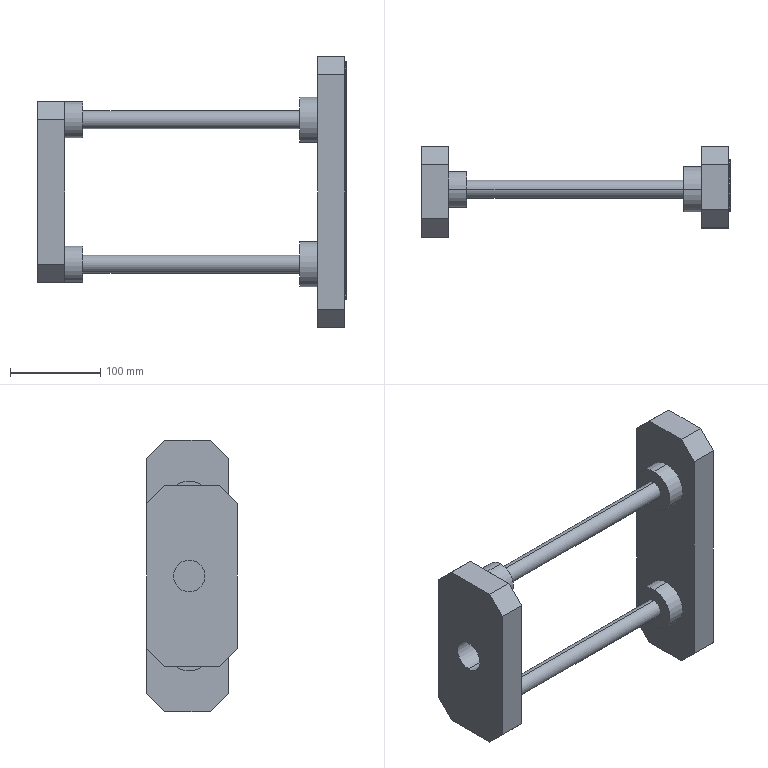Part | STEP file | Blocking plate | 2 solids | 176 faces | box 341.5 x 100 x 300 mm | volume 1615392 mm3 | plane 58 | spline 56 | cylinder 54 | torus 8 | commonest cylinder face diameters 1 x32 20 x4 40 x4 50 x4 6 x3 12 x2